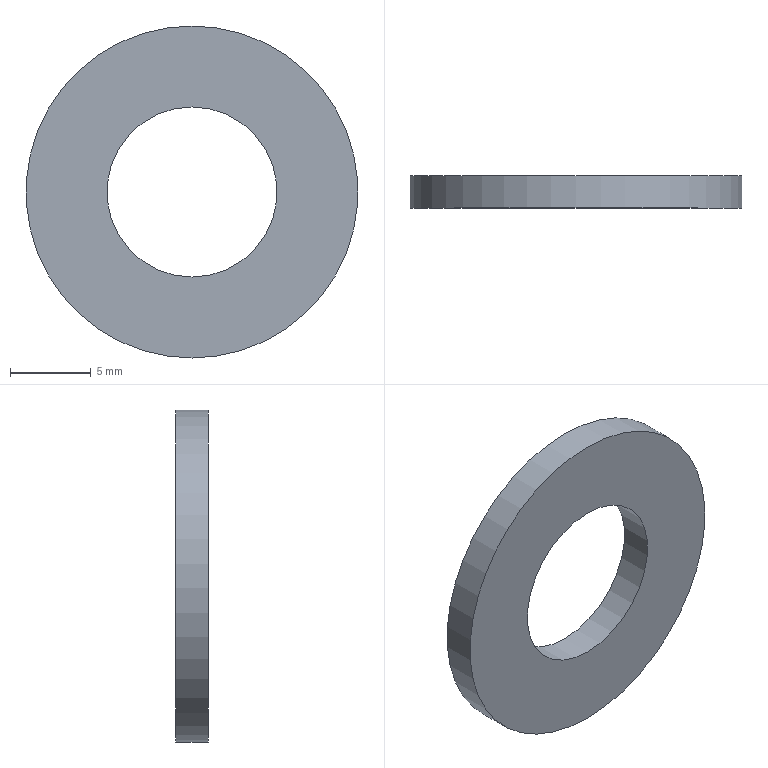Part | NX | features solid 2 | 1 solid | 4 faces | box 20.5 x 2 x 20.5 mm | volume 486.947 mm3 | cylinder 2 | plane 2 | commonest cylinder face diameters 10.5 x1 20.5 x1
STEP:
#1=CARTESIAN_POINT('',(905.,-71.,-63.75));
#2=VERTEX_POINT('',#1);
#3=CARTESIAN_POINT('',(905.,-71.,-74.));
#4=DIRECTION('',(0.,1.,0.));
#5=DIRECTION('',(0.,0.,1.));
#6=AXIS2_PLACEMENT_3D('',#3,#4,#5);
#7=CIRCLE('',#6,10.25);
#8=EDGE_CURVE('',#2,#2,#7,.F.);
#9=ORIENTED_EDGE('',*,*,#8,.T.);
#10=EDGE_LOOP('',(#9));
#11=FACE_BOUND('',#10,.T.);
#12=CARTESIAN_POINT('',(905.,-73.,-63.75));
#13=VERTEX_POINT('',#12);
#14=CARTESIAN_POINT('',(905.,-73.,-74.));
#15=DIRECTION('',(0.,1.,0.));
#16=DIRECTION('',(0.,0.,1.));
#17=AXIS2_PLACEMENT_3D('',#14,#15,#16);
#18=CIRCLE('',#17,10.25);
#19=EDGE_CURVE('',#13,#13,#18,.F.);
#20=ORIENTED_EDGE('',*,*,#19,.F.);
#21=EDGE_LOOP('',(#20));
#22=FACE_BOUND('',#21,.T.);
#23=CARTESIAN_POINT('',(905.,-73.,-74.));
#24=DIRECTION('',(0.,1.,0.));
#25=DIRECTION('',(0.,0.,1.));
#26=AXIS2_PLACEMENT_3D('',#23,#24,#25);
#27=CYLINDRICAL_SURFACE('',#26,10.25);
#28=ADVANCED_FACE('',(#11,#22),#27,.T.);
#29=ORIENTED_EDGE('',*,*,#19,.T.);
#30=EDGE_LOOP('',(#29));
#31=FACE_BOUND('',#30,.T.);
#32=CARTESIAN_POINT('',(905.,-73.,-79.25));
#33=VERTEX_POINT('',#32);
#34=CARTESIAN_POINT('',(905.,-73.,-74.));
#35=DIRECTION('',(0.,-1.,0.));
#36=DIRECTION('',(0.,0.,-1.));
#37=AXIS2_PLACEMENT_3D('',#34,#35,#36);
#38=CIRCLE('',#37,5.25);
#39=EDGE_CURVE('',#33,#33,#38,.T.);
#40=ORIENTED_EDGE('',*,*,#39,.F.);
#41=EDGE_LOOP('',(#40));
#42=FACE_BOUND('',#41,.T.);
#43=CARTESIAN_POINT('',(905.,-73.,-74.));
#44=DIRECTION('',(0.,1.,0.));
#45=DIRECTION('',(0.,0.,1.));
#46=AXIS2_PLACEMENT_3D('',#43,#44,#45);
#47=PLANE('',#46);
#48=ADVANCED_FACE('',(#31,#42),#47,.F.);
#49=ORIENTED_EDGE('',*,*,#8,.F.);
#50=EDGE_LOOP('',(#49));
#51=FACE_BOUND('',#50,.T.);
#52=CARTESIAN_POINT('',(905.,-71.,-79.25));
#53=VERTEX_POINT('',#52);
#54=CARTESIAN_POINT('',(905.,-71.,-74.));
#55=DIRECTION('',(0.,-1.,0.));
#56=DIRECTION('',(0.,0.,-1.));
#57=AXIS2_PLACEMENT_3D('',#54,#55,#56);
#58=CIRCLE('',#57,5.25);
#59=EDGE_CURVE('',#53,#53,#58,.T.);
#60=ORIENTED_EDGE('',*,*,#59,.T.);
#61=EDGE_LOOP('',(#60));
#62=FACE_BOUND('',#61,.T.);
#63=CARTESIAN_POINT('',(905.,-71.,-74.));
#64=DIRECTION('',(0.,1.,0.));
#65=DIRECTION('',(0.,0.,1.));
#66=AXIS2_PLACEMENT_3D('',#63,#64,#65);
#67=PLANE('',#66);
#68=ADVANCED_FACE('',(#51,#62),#67,.T.);
#69=ORIENTED_EDGE('',*,*,#59,.F.);
#70=EDGE_LOOP('',(#69));
#71=FACE_BOUND('',#70,.T.);
#72=ORIENTED_EDGE('',*,*,#39,.T.);
#73=EDGE_LOOP('',(#72));
#74=FACE_BOUND('',#73,.T.);
#75=CARTESIAN_POINT('',(905.,-73.,-74.));
#76=DIRECTION('',(0.,1.,0.));
#77=DIRECTION('',(0.,0.,1.));
#78=AXIS2_PLACEMENT_3D('',#75,#76,#77);
#79=CYLINDRICAL_SURFACE('',#78,5.25);
#80=ADVANCED_FACE('',(#71,#74),#79,.F.);
#81=CLOSED_SHELL('',(#28,#48,#68,#80));
#82=MANIFOLD_SOLID_BREP('',#81);
#83=(LENGTH_UNIT()NAMED_UNIT(*)SI_UNIT(.MILLI.,.METRE.));
#84=UNCERTAINTY_MEASURE_WITH_UNIT(LENGTH_MEASURE(0.00001),#83,'','');
#85=(NAMED_UNIT(*)PLANE_ANGLE_UNIT()SI_UNIT($,.RADIAN.));
#86=(NAMED_UNIT(*)SI_UNIT($,.STERADIAN.)SOLID_ANGLE_UNIT());
#87=(GEOMETRIC_REPRESENTATION_CONTEXT(3)GLOBAL_UNCERTAINTY_ASSIGNED_CONTEXT((#84))GLOBAL_UNIT_ASSIGNED_CONTEXT((#83,#85,#86))REPRESENTATION_CONTEXT('',''));
#88=ADVANCED_BREP_SHAPE_REPRESENTATION('',(#82),#87);